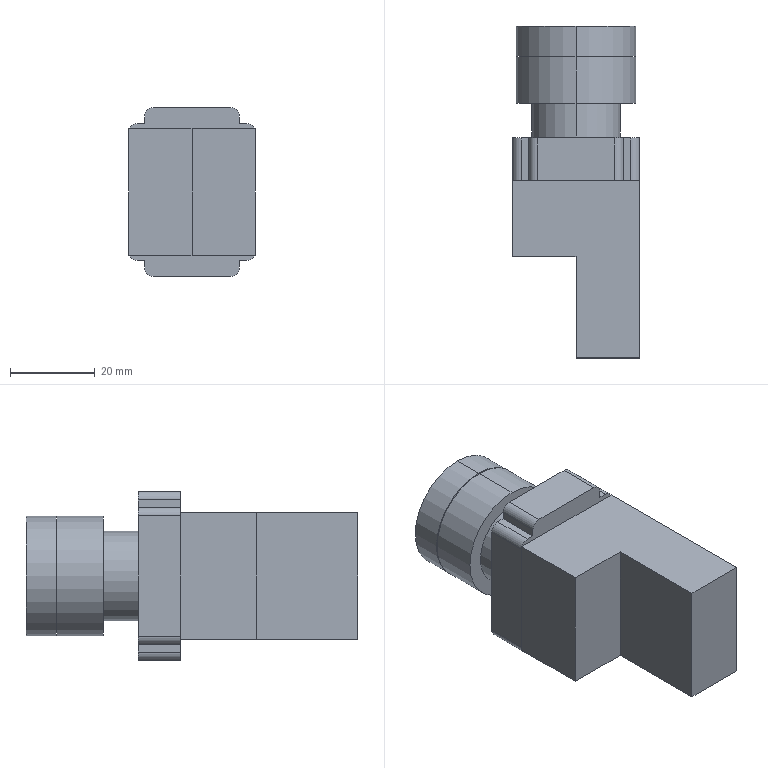Part | SolidWorks | features Boss 3, Revolution 2, Cut 1, Fillet 1 | 4 solids | 46 faces | box 30 x 78.5 x 40 mm | volume 52539 mm3 | plane 28 | cylinder 18 | commonest cylinder face diameters 4 x8 28.2 x4 21.2 x2 25 x2 25.4 x2
STEP:
#1=CARTESIAN_POINT('',(0.,8.2,-10.6));
#2=VERTEX_POINT('',#1);
#3=CARTESIAN_POINT('',(0.,8.2,10.6));
#4=VERTEX_POINT('',#3);
#5=CARTESIAN_POINT('',(0.,8.2,0.));
#6=DIRECTION('',(0.,-1.,0.));
#7=DIRECTION('',(0.,0.,-1.));
#8=AXIS2_PLACEMENT_3D('',#5,#6,#7);
#9=CIRCLE('',#8,10.6);
#10=EDGE_CURVE('',#2,#4,#9,.T.);
#11=ORIENTED_EDGE('',*,*,#10,.T.);
#12=CARTESIAN_POINT('',(0.,0.,10.6));
#13=VERTEX_POINT('',#12);
#14=CARTESIAN_POINT('',(0.,0.,10.6));
#15=DIRECTION('',(0.,-1.,0.));
#16=VECTOR('',#15,1000.);
#17=LINE('',#14,#16);
#18=EDGE_CURVE('',#4,#13,#17,.T.);
#19=ORIENTED_EDGE('',*,*,#18,.T.);
#20=CARTESIAN_POINT('',(0.,0.,-10.6));
#21=VERTEX_POINT('',#20);
#22=CARTESIAN_POINT('',(0.,0.,0.));
#23=DIRECTION('',(0.,-1.,0.));
#24=DIRECTION('',(0.,0.,-1.));
#25=AXIS2_PLACEMENT_3D('',#22,#23,#24);
#26=CIRCLE('',#25,10.6);
#27=EDGE_CURVE('',#21,#13,#26,.T.);
#28=ORIENTED_EDGE('',*,*,#27,.F.);
#29=CARTESIAN_POINT('',(0.,0.,-10.6));
#30=DIRECTION('',(0.,-1.,0.));
#31=VECTOR('',#30,1000.);
#32=LINE('',#29,#31);
#33=EDGE_CURVE('',#2,#21,#32,.T.);
#34=ORIENTED_EDGE('',*,*,#33,.F.);
#35=EDGE_LOOP('',(#11,#19,#28,#34));
#36=FACE_OUTER_BOUND('',#35,.T.);
#37=CARTESIAN_POINT('',(0.,0.,0.));
#38=DIRECTION('',(0.,-1.,0.));
#39=DIRECTION('',(0.,0.,-1.));
#40=AXIS2_PLACEMENT_3D('',#37,#38,#39);
#41=CYLINDRICAL_SURFACE('',#40,10.6);
#42=ADVANCED_FACE('',(#36),#41,.T.);
#43=CARTESIAN_POINT('',(0.,19.2,-14.1));
#44=VERTEX_POINT('',#43);
#45=CARTESIAN_POINT('',(0.,19.2,14.1));
#46=VERTEX_POINT('',#45);
#47=CARTESIAN_POINT('',(0.,19.2,0.));
#48=DIRECTION('',(0.,-1.,0.));
#49=DIRECTION('',(0.,0.,-1.));
#50=AXIS2_PLACEMENT_3D('',#47,#48,#49);
#51=CIRCLE('',#50,14.1);
#52=EDGE_CURVE('',#44,#46,#51,.T.);
#53=ORIENTED_EDGE('',*,*,#52,.T.);
#54=CARTESIAN_POINT('',(0.,8.2,14.1));
#55=VERTEX_POINT('',#54);
#56=CARTESIAN_POINT('',(0.,0.,14.1));
#57=DIRECTION('',(0.,-1.,0.));
#58=VECTOR('',#57,1000.);
#59=LINE('',#56,#58);
#60=EDGE_CURVE('',#46,#55,#59,.T.);
#61=ORIENTED_EDGE('',*,*,#60,.T.);
#62=CARTESIAN_POINT('',(0.,8.2,-14.1));
#63=VERTEX_POINT('',#62);
#64=CARTESIAN_POINT('',(0.,8.2,0.));
#65=DIRECTION('',(0.,-1.,0.));
#66=DIRECTION('',(0.,0.,-1.));
#67=AXIS2_PLACEMENT_3D('',#64,#65,#66);
#68=CIRCLE('',#67,14.1);
#69=EDGE_CURVE('',#63,#55,#68,.T.);
#70=ORIENTED_EDGE('',*,*,#69,.F.);
#71=CARTESIAN_POINT('',(0.,0.,-14.1));
#72=DIRECTION('',(0.,-1.,0.));
#73=VECTOR('',#72,1000.);
#74=LINE('',#71,#73);
#75=EDGE_CURVE('',#44,#63,#74,.T.);
#76=ORIENTED_EDGE('',*,*,#75,.F.);
#77=EDGE_LOOP('',(#53,#61,#70,#76));
#78=FACE_OUTER_BOUND('',#77,.T.);
#79=CARTESIAN_POINT('',(0.,0.,0.));
#80=DIRECTION('',(0.,-1.,0.));
#81=DIRECTION('',(0.,0.,-1.));
#82=AXIS2_PLACEMENT_3D('',#79,#80,#81);
#83=CYLINDRICAL_SURFACE('',#82,14.1);
#84=ADVANCED_FACE('',(#78),#83,.T.);
#85=CARTESIAN_POINT('',(0.,26.5,-12.5));
#86=VERTEX_POINT('',#85);
#87=CARTESIAN_POINT('',(0.,26.5,12.5));
#88=VERTEX_POINT('',#87);
#89=CARTESIAN_POINT('',(0.,26.5,0.));
#90=DIRECTION('',(0.,-1.,0.));
#91=DIRECTION('',(0.,0.,-1.));
#92=AXIS2_PLACEMENT_3D('',#89,#90,#91);
#93=CIRCLE('',#92,12.5);
#94=EDGE_CURVE('',#86,#88,#93,.T.);
#95=ORIENTED_EDGE('',*,*,#94,.T.);
#96=CARTESIAN_POINT('',(0.,19.2,12.5));
#97=VERTEX_POINT('',#96);
#98=CARTESIAN_POINT('',(0.,0.,12.5));
#99=DIRECTION('',(0.,-1.,0.));
#100=VECTOR('',#99,1000.);
#101=LINE('',#98,#100);
#102=EDGE_CURVE('',#88,#97,#101,.T.);
#103=ORIENTED_EDGE('',*,*,#102,.T.);
#104=CARTESIAN_POINT('',(0.,19.2,-12.5));
#105=VERTEX_POINT('',#104);
#106=CARTESIAN_POINT('',(0.,19.2,0.));
#107=DIRECTION('',(0.,-1.,0.));
#108=DIRECTION('',(0.,0.,-1.));
#109=AXIS2_PLACEMENT_3D('',#106,#107,#108);
#110=CIRCLE('',#109,12.5);
#111=EDGE_CURVE('',#105,#97,#110,.T.);
#112=ORIENTED_EDGE('',*,*,#111,.F.);
#113=CARTESIAN_POINT('',(0.,0.,-12.5));
#114=DIRECTION('',(0.,-1.,0.));
#115=VECTOR('',#114,1000.);
#116=LINE('',#113,#115);
#117=EDGE_CURVE('',#86,#105,#116,.T.);
#118=ORIENTED_EDGE('',*,*,#117,.F.);
#119=EDGE_LOOP('',(#95,#103,#112,#118));
#120=FACE_OUTER_BOUND('',#119,.T.);
#121=CARTESIAN_POINT('',(0.,0.,0.));
#122=DIRECTION('',(0.,-1.,0.));
#123=DIRECTION('',(0.,0.,-1.));
#124=AXIS2_PLACEMENT_3D('',#121,#122,#123);
#125=CYLINDRICAL_SURFACE('',#124,12.5);
#126=ADVANCED_FACE('',(#120),#125,.T.);
#127=ORIENTED_EDGE('',*,*,#27,.T.);
#128=CARTESIAN_POINT('',(0.,0.,0.));
#129=DIRECTION('',(0.,-1.,0.));
#130=DIRECTION('',(0.,0.,-1.));
#131=AXIS2_PLACEMENT_3D('',#128,#129,#130);
#132=CIRCLE('',#131,10.6);
#133=EDGE_CURVE('',#13,#21,#132,.T.);
#134=ORIENTED_EDGE('',*,*,#133,.T.);
#135=EDGE_LOOP('',(#127,#134));
#136=FACE_OUTER_BOUND('',#135,.T.);
#137=CARTESIAN_POINT('',(10.6,0.,0.));
#138=DIRECTION('',(0.,-1.,0.));
#139=DIRECTION('',(0.,0.,-1.));
#140=AXIS2_PLACEMENT_3D('',#137,#138,#139);
#141=PLANE('',#140);
#142=ADVANCED_FACE('',(#136),#141,.T.);
#143=ORIENTED_EDGE('',*,*,#94,.F.);
#144=CARTESIAN_POINT('',(0.,26.5,0.));
#145=DIRECTION('',(0.,-1.,0.));
#146=DIRECTION('',(0.,0.,-1.));
#147=AXIS2_PLACEMENT_3D('',#144,#145,#146);
#148=CIRCLE('',#147,12.5);
#149=EDGE_CURVE('',#88,#86,#148,.T.);
#150=ORIENTED_EDGE('',*,*,#149,.F.);
#151=EDGE_LOOP('',(#143,#150));
#152=FACE_OUTER_BOUND('',#151,.T.);
#153=CARTESIAN_POINT('',(0.,26.5,0.));
#154=DIRECTION('',(0.,1.,0.));
#155=DIRECTION('',(0.,0.,1.));
#156=AXIS2_PLACEMENT_3D('',#153,#154,#155);
#157=PLANE('',#156);
#158=ADVANCED_FACE('',(#152),#157,.T.);
#159=ORIENTED_EDGE('',*,*,#102,.F.);
#160=ORIENTED_EDGE('',*,*,#149,.T.);
#161=ORIENTED_EDGE('',*,*,#117,.T.);
#162=CARTESIAN_POINT('',(0.,19.2,0.));
#163=DIRECTION('',(0.,-1.,0.));
#164=DIRECTION('',(0.,0.,-1.));
#165=AXIS2_PLACEMENT_3D('',#162,#163,#164);
#166=CIRCLE('',#165,12.5);
#167=EDGE_CURVE('',#97,#105,#166,.T.);
#168=ORIENTED_EDGE('',*,*,#167,.F.);
#169=EDGE_LOOP('',(#159,#160,#161,#168));
#170=FACE_OUTER_BOUND('',#169,.T.);
#171=CARTESIAN_POINT('',(0.,0.,0.));
#172=DIRECTION('',(0.,-1.,0.));
#173=DIRECTION('',(0.,0.,-1.));
#174=AXIS2_PLACEMENT_3D('',#171,#172,#173);
#175=CYLINDRICAL_SURFACE('',#174,12.5);
#176=ADVANCED_FACE('',(#170),#175,.T.);
#177=ORIENTED_EDGE('',*,*,#111,.T.);
#178=ORIENTED_EDGE('',*,*,#167,.T.);
#179=EDGE_LOOP('',(#177,#178));
#180=FACE_BOUND('',#179,.T.);
#181=ORIENTED_EDGE('',*,*,#52,.F.);
#182=CARTESIAN_POINT('',(0.,19.2,0.));
#183=DIRECTION('',(0.,-1.,0.));
#184=DIRECTION('',(0.,0.,-1.));
#185=AXIS2_PLACEMENT_3D('',#182,#183,#184);
#186=CIRCLE('',#185,14.1);
#187=EDGE_CURVE('',#46,#44,#186,.T.);
#188=ORIENTED_EDGE('',*,*,#187,.F.);
#189=EDGE_LOOP('',(#181,#188));
#190=FACE_OUTER_BOUND('',#189,.T.);
#191=CARTESIAN_POINT('',(12.5,19.2,0.));
#192=DIRECTION('',(0.,1.,0.));
#193=DIRECTION('',(0.,0.,1.));
#194=AXIS2_PLACEMENT_3D('',#191,#192,#193);
#195=PLANE('',#194);
#196=ADVANCED_FACE('',(#180,#190),#195,.T.);
#197=ORIENTED_EDGE('',*,*,#60,.F.);
#198=ORIENTED_EDGE('',*,*,#187,.T.);
#199=ORIENTED_EDGE('',*,*,#75,.T.);
#200=CARTESIAN_POINT('',(0.,8.2,0.));
#201=DIRECTION('',(0.,-1.,0.));
#202=DIRECTION('',(0.,0.,-1.));
#203=AXIS2_PLACEMENT_3D('',#200,#201,#202);
#204=CIRCLE('',#203,14.1);
#205=EDGE_CURVE('',#55,#63,#204,.T.);
#206=ORIENTED_EDGE('',*,*,#205,.F.);
#207=EDGE_LOOP('',(#197,#198,#199,#206));
#208=FACE_OUTER_BOUND('',#207,.T.);
#209=CARTESIAN_POINT('',(0.,0.,0.));
#210=DIRECTION('',(0.,-1.,0.));
#211=DIRECTION('',(0.,0.,-1.));
#212=AXIS2_PLACEMENT_3D('',#209,#210,#211);
#213=CYLINDRICAL_SURFACE('',#212,14.1);
#214=ADVANCED_FACE('',(#208),#213,.T.);
#215=ORIENTED_EDGE('',*,*,#69,.T.);
#216=ORIENTED_EDGE('',*,*,#205,.T.);
#217=EDGE_LOOP('',(#215,#216));
#218=FACE_OUTER_BOUND('',#217,.T.);
#219=ORIENTED_EDGE('',*,*,#10,.F.);
#220=CARTESIAN_POINT('',(0.,8.2,0.));
#221=DIRECTION('',(0.,-1.,0.));
#222=DIRECTION('',(0.,0.,-1.));
#223=AXIS2_PLACEMENT_3D('',#220,#221,#222);
#224=CIRCLE('',#223,10.6);
#225=EDGE_CURVE('',#4,#2,#224,.T.);
#226=ORIENTED_EDGE('',*,*,#225,.F.);
#227=EDGE_LOOP('',(#219,#226));
#228=FACE_BOUND('',#227,.T.);
#229=CARTESIAN_POINT('',(14.1,8.2,0.));
#230=DIRECTION('',(0.,-1.,0.));
#231=DIRECTION('',(0.,0.,-1.));
#232=AXIS2_PLACEMENT_3D('',#229,#230,#231);
#233=PLANE('',#232);
#234=ADVANCED_FACE('',(#218,#228),#233,.T.);
#235=ORIENTED_EDGE('',*,*,#18,.F.);
#236=ORIENTED_EDGE('',*,*,#225,.T.);
#237=ORIENTED_EDGE('',*,*,#33,.T.);
#238=ORIENTED_EDGE('',*,*,#133,.F.);
#239=EDGE_LOOP('',(#235,#236,#237,#238));
#240=FACE_OUTER_BOUND('',#239,.T.);
#241=CARTESIAN_POINT('',(0.,0.,0.));
#242=DIRECTION('',(0.,-1.,0.));
#243=DIRECTION('',(0.,0.,-1.));
#244=AXIS2_PLACEMENT_3D('',#241,#242,#243);
#245=CYLINDRICAL_SURFACE('',#244,10.6);
#246=ADVANCED_FACE('',(#240),#245,.T.);
#247=CLOSED_SHELL('',(#42,#84,#126,#142,#158,#176,#196,#214,#234,#246));
#248=MANIFOLD_SOLID_BREP('',#247);
#249=CARTESIAN_POINT('',(15.,0.,-14.2));
#250=VERTEX_POINT('',#249);
#251=CARTESIAN_POINT('',(15.,0.,14.2));
#252=VERTEX_POINT('',#251);
#253=CARTESIAN_POINT('',(15.,0.,20.));
#254=DIRECTION('',(0.,0.,1.));
#255=VECTOR('',#254,1000.);
#256=LINE('',#253,#255);
#257=EDGE_CURVE('',#250,#252,#256,.T.);
#258=ORIENTED_EDGE('',*,*,#257,.T.);
#259=CARTESIAN_POINT('',(15.,-10.,14.2));
#260=VERTEX_POINT('',#259);
#261=CARTESIAN_POINT('',(15.,-10.,14.2));
#262=DIRECTION('',(0.,-1.,0.));
#263=VECTOR('',#262,1000.);
#264=LINE('',#261,#263);
#265=EDGE_CURVE('',#252,#260,#264,.T.);
#266=ORIENTED_EDGE('',*,*,#265,.T.);
#267=CARTESIAN_POINT('',(15.,-10.,-14.2));
#268=VERTEX_POINT('',#267);
#269=CARTESIAN_POINT('',(15.,-10.,20.));
#270=DIRECTION('',(0.,0.,1.));
#271=VECTOR('',#270,1000.);
#272=LINE('',#269,#271);
#273=EDGE_CURVE('',#268,#260,#272,.T.);
#274=ORIENTED_EDGE('',*,*,#273,.F.);
#275=CARTESIAN_POINT('',(15.,-10.,-14.2));
#276=DIRECTION('',(0.,1.,0.));
#277=VECTOR('',#276,1000.);
#278=LINE('',#275,#277);
#279=EDGE_CURVE('',#268,#250,#278,.T.);
#280=ORIENTED_EDGE('',*,*,#279,.T.);
#281=EDGE_LOOP('',(#258,#266,#274,#280));
#282=FACE_OUTER_BOUND('',#281,.T.);
#283=CARTESIAN_POINT('',(15.,-10.,20.));
#284=DIRECTION('',(-1.,0.,0.));
#285=DIRECTION('',(0.,0.,1.));
#286=AXIS2_PLACEMENT_3D('',#283,#284,#285);
#287=PLANE('',#286);
#288=ADVANCED_FACE('',(#282),#287,.F.);
#289=CARTESIAN_POINT('',(9.2,0.,20.));
#290=VERTEX_POINT('',#289);
#291=CARTESIAN_POINT('',(-9.2,0.,20.));
#292=VERTEX_POINT('',#291);
#293=CARTESIAN_POINT('',(15.,0.,20.));
#294=DIRECTION('',(-1.,0.,0.));
#295=VECTOR('',#294,1000.);
#296=LINE('',#293,#295);
#297=EDGE_CURVE('',#290,#292,#296,.T.);
#298=ORIENTED_EDGE('',*,*,#297,.T.);
#299=CARTESIAN_POINT('',(-9.2,-10.,20.));
#300=VERTEX_POINT('',#299);
#301=CARTESIAN_POINT('',(-9.2,-10.,20.));
#302=DIRECTION('',(0.,-1.,0.));
#303=VECTOR('',#302,1000.);
#304=LINE('',#301,#303);
#305=EDGE_CURVE('',#292,#300,#304,.T.);
#306=ORIENTED_EDGE('',*,*,#305,.T.);
#307=CARTESIAN_POINT('',(9.2,-10.,20.));
#308=VERTEX_POINT('',#307);
#309=CARTESIAN_POINT('',(15.,-10.,20.));
#310=DIRECTION('',(-1.,0.,0.));
#311=VECTOR('',#310,1000.);
#312=LINE('',#309,#311);
#313=EDGE_CURVE('',#308,#300,#312,.T.);
#314=ORIENTED_EDGE('',*,*,#313,.F.);
#315=CARTESIAN_POINT('',(9.2,-10.,20.));
#316=DIRECTION('',(0.,1.,0.));
#317=VECTOR('',#316,1000.);
#318=LINE('',#315,#317);
#319=EDGE_CURVE('',#308,#290,#318,.T.);
#320=ORIENTED_EDGE('',*,*,#319,.T.);
#321=EDGE_LOOP('',(#298,#306,#314,#320));
#322=FACE_OUTER_BOUND('',#321,.T.);
#323=CARTESIAN_POINT('',(15.,-10.,20.));
#324=DIRECTION('',(0.,0.,-1.));
#325=DIRECTION('',(-1.,0.,0.));
#326=AXIS2_PLACEMENT_3D('',#323,#324,#325);
#327=PLANE('',#326);
#328=ADVANCED_FACE('',(#322),#327,.F.);
#329=CARTESIAN_POINT('',(-15.,-10.,14.2));
#330=VERTEX_POINT('',#329);
#331=CARTESIAN_POINT('',(-15.,-10.,-14.2));
#332=VERTEX_POINT('',#331);
#333=CARTESIAN_POINT('',(-15.,-10.,20.));
#334=DIRECTION('',(0.,0.,-1.));
#335=VECTOR('',#334,1000.);
#336=LINE('',#333,#335);
#337=EDGE_CURVE('',#330,#332,#336,.T.);
#338=ORIENTED_EDGE('',*,*,#337,.F.);
#339=CARTESIAN_POINT('',(-15.,0.,14.2));
#340=VERTEX_POINT('',#339);
#341=CARTESIAN_POINT('',(-15.,-10.,14.2));
#342=DIRECTION('',(0.,1.,0.));
#343=VECTOR('',#342,1000.);
#344=LINE('',#341,#343);
#345=EDGE_CURVE('',#330,#340,#344,.T.);
#346=ORIENTED_EDGE('',*,*,#345,.T.);
#347=CARTESIAN_POINT('',(-15.,0.,-14.2));
#348=VERTEX_POINT('',#347);
#349=CARTESIAN_POINT('',(-15.,0.,20.));
#350=DIRECTION('',(0.,0.,-1.));
#351=VECTOR('',#350,1000.);
#352=LINE('',#349,#351);
#353=EDGE_CURVE('',#340,#348,#352,.T.);
#354=ORIENTED_EDGE('',*,*,#353,.T.);
#355=CARTESIAN_POINT('',(-15.,-10.,-14.2));
#356=DIRECTION('',(0.,-1.,0.));
#357=VECTOR('',#356,1000.);
#358=LINE('',#355,#357);
#359=EDGE_CURVE('',#348,#332,#358,.T.);
#360=ORIENTED_EDGE('',*,*,#359,.T.);
#361=EDGE_LOOP('',(#338,#346,#354,#360));
#362=FACE_OUTER_BOUND('',#361,.T.);
#363=CARTESIAN_POINT('',(-15.,-10.,20.));
#364=DIRECTION('',(1.,0.,0.));
#365=DIRECTION('',(0.,0.,-1.));
#366=AXIS2_PLACEMENT_3D('',#363,#364,#365);
#367=PLANE('',#366);
#368=ADVANCED_FACE('',(#362),#367,.F.);
#369=CARTESIAN_POINT('',(-9.2,0.,-20.));
#370=VERTEX_POINT('',#369);
#371=CARTESIAN_POINT('',(9.2,0.,-20.));
#372=VERTEX_POINT('',#371);
#373=CARTESIAN_POINT('',(15.,0.,-20.));
#374=DIRECTION('',(1.,0.,0.));
#375=VECTOR('',#374,1000.);
#376=LINE('',#373,#375);
#377=EDGE_CURVE('',#370,#372,#376,.T.);
#378=ORIENTED_EDGE('',*,*,#377,.T.);
#379=CARTESIAN_POINT('',(9.2,-10.,-20.));
#380=VERTEX_POINT('',#379);
#381=CARTESIAN_POINT('',(9.2,-10.,-20.));
#382=DIRECTION('',(0.,-1.,0.));
#383=VECTOR('',#382,1000.);
#384=LINE('',#381,#383);
#385=EDGE_CURVE('',#372,#380,#384,.T.);
#386=ORIENTED_EDGE('',*,*,#385,.T.);
#387=CARTESIAN_POINT('',(-9.2,-10.,-20.));
#388=VERTEX_POINT('',#387);
#389=CARTESIAN_POINT('',(15.,-10.,-20.));
#390=DIRECTION('',(1.,0.,0.));
#391=VECTOR('',#390,1000.);
#392=LINE('',#389,#391);
#393=EDGE_CURVE('',#388,#380,#392,.T.);
#394=ORIENTED_EDGE('',*,*,#393,.F.);
#395=CARTESIAN_POINT('',(-9.2,-10.,-20.));
#396=DIRECTION('',(0.,1.,0.));
#397=VECTOR('',#396,1000.);
#398=LINE('',#395,#397);
#399=EDGE_CURVE('',#388,#370,#398,.T.);
#400=ORIENTED_EDGE('',*,*,#399,.T.);
#401=EDGE_LOOP('',(#378,#386,#394,#400));
#402=FACE_OUTER_BOUND('',#401,.T.);
#403=CARTESIAN_POINT('',(15.,-10.,-20.));
#404=DIRECTION('',(0.,0.,1.));
#405=DIRECTION('',(1.,0.,0.));
#406=AXIS2_PLACEMENT_3D('',#403,#404,#405);
#407=PLANE('',#406);
#408=ADVANCED_FACE('',(#402),#407,.F.);
#409=CARTESIAN_POINT('',(-13.,-10.,16.2));
#410=VERTEX_POINT('',#409);
#411=CARTESIAN_POINT('',(-11.2,-10.,16.2));
#412=VERTEX_POINT('',#411);
#413=CARTESIAN_POINT('',(-15.,-10.,16.2));
#414=DIRECTION('',(1.,0.,0.));
#415=VECTOR('',#414,1000.);
#416=LINE('',#413,#415);
#417=EDGE_CURVE('',#410,#412,#416,.T.);
#418=ORIENTED_EDGE('',*,*,#417,.F.);
#419=CARTESIAN_POINT('',(-13.,-10.,14.2));
#420=DIRECTION('',(0.,-1.,0.));
#421=DIRECTION('',(0.,0.,1.));
#422=AXIS2_PLACEMENT_3D('',#419,#420,#421);
#423=CIRCLE('',#422,2.);
#424=EDGE_CURVE('',#410,#330,#423,.T.);
#425=ORIENTED_EDGE('',*,*,#424,.T.);
#426=ORIENTED_EDGE('',*,*,#337,.T.);
#427=CARTESIAN_POINT('',(-13.,-10.,-16.2));
#428=VERTEX_POINT('',#427);
#429=CARTESIAN_POINT('',(-13.,-10.,-14.2));
#430=DIRECTION('',(0.,-1.,0.));
#431=DIRECTION('',(0.,0.,1.));
#432=AXIS2_PLACEMENT_3D('',#429,#430,#431);
#433=CIRCLE('',#432,2.);
#434=EDGE_CURVE('',#332,#428,#433,.T.);
#435=ORIENTED_EDGE('',*,*,#434,.T.);
#436=CARTESIAN_POINT('',(-11.2,-10.,-16.2));
#437=VERTEX_POINT('',#436);
#438=CARTESIAN_POINT('',(-15.,-10.,-16.2));
#439=DIRECTION('',(-1.,0.,0.));
#440=VECTOR('',#439,1000.);
#441=LINE('',#438,#440);
#442=EDGE_CURVE('',#437,#428,#441,.T.);
#443=ORIENTED_EDGE('',*,*,#442,.F.);
#444=CARTESIAN_POINT('',(-11.2,-10.,-18.));
#445=VERTEX_POINT('',#444);
#446=CARTESIAN_POINT('',(-11.2,-10.,-20.));
#447=DIRECTION('',(0.,0.,1.));
#448=VECTOR('',#447,1000.);
#449=LINE('',#446,#448);
#450=EDGE_CURVE('',#445,#437,#449,.T.);
#451=ORIENTED_EDGE('',*,*,#450,.F.);
#452=CARTESIAN_POINT('',(-9.2,-10.,-18.));
#453=DIRECTION('',(0.,-1.,0.));
#454=DIRECTION('',(0.,0.,1.));
#455=AXIS2_PLACEMENT_3D('',#452,#453,#454);
#456=CIRCLE('',#455,2.);
#457=EDGE_CURVE('',#445,#388,#456,.T.);
#458=ORIENTED_EDGE('',*,*,#457,.T.);
#459=ORIENTED_EDGE('',*,*,#393,.T.);
#460=CARTESIAN_POINT('',(11.2,-10.,-18.));
#461=VERTEX_POINT('',#460);
#462=CARTESIAN_POINT('',(9.2,-10.,-18.));
#463=DIRECTION('',(0.,-1.,0.));
#464=DIRECTION('',(0.,0.,1.));
#465=AXIS2_PLACEMENT_3D('',#462,#463,#464);
#466=CIRCLE('',#465,2.);
#467=EDGE_CURVE('',#380,#461,#466,.T.);
#468=ORIENTED_EDGE('',*,*,#467,.T.);
#469=CARTESIAN_POINT('',(11.2,-10.,-16.2));
#470=VERTEX_POINT('',#469);
#471=CARTESIAN_POINT('',(11.2,-10.,-20.));
#472=DIRECTION('',(0.,0.,-1.));
#473=VECTOR('',#472,1000.);
#474=LINE('',#471,#473);
#475=EDGE_CURVE('',#470,#461,#474,.T.);
#476=ORIENTED_EDGE('',*,*,#475,.F.);
#477=CARTESIAN_POINT('',(13.,-10.,-16.2));
#478=VERTEX_POINT('',#477);
#479=CARTESIAN_POINT('',(15.,-10.,-16.2));
#480=DIRECTION('',(-1.,0.,0.));
#481=VECTOR('',#480,1000.);
#482=LINE('',#479,#481);
#483=EDGE_CURVE('',#478,#470,#482,.T.);
#484=ORIENTED_EDGE('',*,*,#483,.F.);
#485=CARTESIAN_POINT('',(13.,-10.,-14.2));
#486=DIRECTION('',(0.,-1.,0.));
#487=DIRECTION('',(0.,0.,1.));
#488=AXIS2_PLACEMENT_3D('',#485,#486,#487);
#489=CIRCLE('',#488,2.);
#490=EDGE_CURVE('',#478,#268,#489,.T.);
#491=ORIENTED_EDGE('',*,*,#490,.T.);
#492=ORIENTED_EDGE('',*,*,#273,.T.);
#493=CARTESIAN_POINT('',(13.,-10.,16.2));
#494=VERTEX_POINT('',#493);
#495=CARTESIAN_POINT('',(13.,-10.,14.2));
#496=DIRECTION('',(0.,-1.,0.));
#497=DIRECTION('',(0.,0.,1.));
#498=AXIS2_PLACEMENT_3D('',#495,#496,#497);
#499=CIRCLE('',#498,2.);
#500=EDGE_CURVE('',#260,#494,#499,.T.);
#501=ORIENTED_EDGE('',*,*,#500,.T.);
#502=CARTESIAN_POINT('',(11.2,-10.,16.2));
#503=VERTEX_POINT('',#502);
#504=CARTESIAN_POINT('',(15.,-10.,16.2));
#505=DIRECTION('',(1.,0.,0.));
#506=VECTOR('',#505,1000.);
#507=LINE('',#504,#506);
#508=EDGE_CURVE('',#503,#494,#507,.T.);
#509=ORIENTED_EDGE('',*,*,#508,.F.);
#510=CARTESIAN_POINT('',(11.2,-10.,18.));
#511=VERTEX_POINT('',#510);
#512=CARTESIAN_POINT('',(11.2,-10.,20.));
#513=DIRECTION('',(0.,0.,-1.));
#514=VECTOR('',#513,1000.);
#515=LINE('',#512,#514);
#516=EDGE_CURVE('',#511,#503,#515,.T.);
#517=ORIENTED_EDGE('',*,*,#516,.F.);
#518=CARTESIAN_POINT('',(9.2,-10.,18.));
#519=DIRECTION('',(0.,-1.,0.));
#520=DIRECTION('',(0.,0.,1.));
#521=AXIS2_PLACEMENT_3D('',#518,#519,#520);
#522=CIRCLE('',#521,2.);
#523=EDGE_CURVE('',#511,#308,#522,.T.);
#524=ORIENTED_EDGE('',*,*,#523,.T.);
#525=ORIENTED_EDGE('',*,*,#313,.T.);
#526=CARTESIAN_POINT('',(-11.2,-10.,18.));
#527=VERTEX_POINT('',#526);
#528=CARTESIAN_POINT('',(-9.2,-10.,18.));
#529=DIRECTION('',(0.,-1.,0.));
#530=DIRECTION('',(0.,0.,1.));
#531=AXIS2_PLACEMENT_3D('',#528,#529,#530);
#532=CIRCLE('',#531,2.);
#533=EDGE_CURVE('',#300,#527,#532,.T.);
#534=ORIENTED_EDGE('',*,*,#533,.T.);
#535=CARTESIAN_POINT('',(-11.2,-10.,20.));
#536=DIRECTION('',(0.,0.,1.));
#537=VECTOR('',#536,1000.);
#538=LINE('',#535,#537);
#539=EDGE_CURVE('',#412,#527,#538,.T.);
#540=ORIENTED_EDGE('',*,*,#539,.F.);
#541=EDGE_LOOP('',(#418,#425,#426,#435,#443,#451,#458,#459,#468,#476,#484,#491,#492,#501,#509,#517,#524,#525,#534,#540));
#542=FACE_OUTER_BOUND('',#541,.T.);
#543=CARTESIAN_POINT('',(15.,-10.,20.));
#544=DIRECTION('',(0.,1.,0.));
#545=DIRECTION('',(0.,0.,1.));
#546=AXIS2_PLACEMENT_3D('',#543,#544,#545);
#547=PLANE('',#546);
#548=ADVANCED_FACE('',(#542),#547,.F.);
#549=ORIENTED_EDGE('',*,*,#353,.F.);
#550=CARTESIAN_POINT('',(-13.,0.,16.2));
#551=VERTEX_POINT('',#550);
#552=CARTESIAN_POINT('',(-13.,0.,14.2));
#553=DIRECTION('',(0.,1.,0.));
#554=DIRECTION('',(0.,0.,1.));
#555=AXIS2_PLACEMENT_3D('',#552,#553,#554);
#556=CIRCLE('',#555,2.);
#557=EDGE_CURVE('',#340,#551,#556,.T.);
#558=ORIENTED_EDGE('',*,*,#557,.T.);
#559=CARTESIAN_POINT('',(-11.2,0.,16.2));
#560=VERTEX_POINT('',#559);
#561=CARTESIAN_POINT('',(-15.,0.,16.2));
#562=DIRECTION('',(-1.,0.,0.));
#563=VECTOR('',#562,1000.);
#564=LINE('',#561,#563);
#565=EDGE_CURVE('',#560,#551,#564,.T.);
#566=ORIENTED_EDGE('',*,*,#565,.F.);
#567=CARTESIAN_POINT('',(-11.2,0.,18.));
#568=VERTEX_POINT('',#567);
#569=CARTESIAN_POINT('',(-11.2,0.,20.));
#570=DIRECTION('',(0.,0.,-1.));
#571=VECTOR('',#570,1000.);
#572=LINE('',#569,#571);
#573=EDGE_CURVE('',#568,#560,#572,.T.);
#574=ORIENTED_EDGE('',*,*,#573,.F.);
#575=CARTESIAN_POINT('',(-9.2,0.,18.));
#576=DIRECTION('',(0.,1.,0.));
#577=DIRECTION('',(0.,0.,1.));
#578=AXIS2_PLACEMENT_3D('',#575,#576,#577);
#579=CIRCLE('',#578,2.);
#580=EDGE_CURVE('',#568,#292,#579,.T.);
#581=ORIENTED_EDGE('',*,*,#580,.T.);
#582=ORIENTED_EDGE('',*,*,#297,.F.);
#583=CARTESIAN_POINT('',(11.2,0.,18.));
#584=VERTEX_POINT('',#583);
#585=CARTESIAN_POINT('',(9.2,0.,18.));
#586=DIRECTION('',(0.,1.,0.));
#587=DIRECTION('',(0.,0.,1.));
#588=AXIS2_PLACEMENT_3D('',#585,#586,#587);
#589=CIRCLE('',#588,2.);
#590=EDGE_CURVE('',#290,#584,#589,.T.);
#591=ORIENTED_EDGE('',*,*,#590,.T.);
#592=CARTESIAN_POINT('',(11.2,0.,16.2));
#593=VERTEX_POINT('',#592);
#594=CARTESIAN_POINT('',(11.2,0.,20.));
#595=DIRECTION('',(0.,0.,1.));
#596=VECTOR('',#595,1000.);
#597=LINE('',#594,#596);
#598=EDGE_CURVE('',#593,#584,#597,.T.);
#599=ORIENTED_EDGE('',*,*,#598,.F.);
#600=CARTESIAN_POINT('',(13.,0.,16.2));
#601=VERTEX_POINT('',#600);
#602=CARTESIAN_POINT('',(15.,0.,16.2));
#603=DIRECTION('',(-1.,0.,0.));
#604=VECTOR('',#603,1000.);
#605=LINE('',#602,#604);
#606=EDGE_CURVE('',#601,#593,#605,.T.);
#607=ORIENTED_EDGE('',*,*,#606,.F.);
#608=CARTESIAN_POINT('',(13.,0.,14.2));
#609=DIRECTION('',(0.,1.,0.));
#610=DIRECTION('',(0.,0.,1.));
#611=AXIS2_PLACEMENT_3D('',#608,#609,#610);
#612=CIRCLE('',#611,2.);
#613=EDGE_CURVE('',#601,#252,#612,.T.);
#614=ORIENTED_EDGE('',*,*,#613,.T.);
#615=ORIENTED_EDGE('',*,*,#257,.F.);
#616=CARTESIAN_POINT('',(13.,0.,-16.2));
#617=VERTEX_POINT('',#616);
#618=CARTESIAN_POINT('',(13.,0.,-14.2));
#619=DIRECTION('',(0.,1.,0.));
#620=DIRECTION('',(0.,0.,1.));
#621=AXIS2_PLACEMENT_3D('',#618,#619,#620);
#622=CIRCLE('',#621,2.);
#623=EDGE_CURVE('',#250,#617,#622,.T.);
#624=ORIENTED_EDGE('',*,*,#623,.T.);
#625=CARTESIAN_POINT('',(11.2,0.,-16.2));
#626=VERTEX_POINT('',#625);
#627=CARTESIAN_POINT('',(15.,0.,-16.2));
#628=DIRECTION('',(1.,0.,0.));
#629=VECTOR('',#628,1000.);
#630=LINE('',#627,#629);
#631=EDGE_CURVE('',#626,#617,#630,.T.);
#632=ORIENTED_EDGE('',*,*,#631,.F.);
#633=CARTESIAN_POINT('',(11.2,0.,-18.));
#634=VERTEX_POINT('',#633);
#635=CARTESIAN_POINT('',(11.2,0.,-20.));
#636=DIRECTION('',(0.,0.,1.));
#637=VECTOR('',#636,1000.);
#638=LINE('',#635,#637);
#639=EDGE_CURVE('',#634,#626,#638,.T.);
#640=ORIENTED_EDGE('',*,*,#639,.F.);
#641=CARTESIAN_POINT('',(9.2,0.,-18.));
#642=DIRECTION('',(0.,1.,0.));
#643=DIRECTION('',(0.,0.,1.));
#644=AXIS2_PLACEMENT_3D('',#641,#642,#643);
#645=CIRCLE('',#644,2.);
#646=EDGE_CURVE('',#634,#372,#645,.T.);
#647=ORIENTED_EDGE('',*,*,#646,.T.);
#648=ORIENTED_EDGE('',*,*,#377,.F.);
#649=CARTESIAN_POINT('',(-11.2,0.,-18.));
#650=VERTEX_POINT('',#649);
#651=CARTESIAN_POINT('',(-9.2,0.,-18.));
#652=DIRECTION('',(0.,1.,0.));
#653=DIRECTION('',(0.,0.,1.));
#654=AXIS2_PLACEMENT_3D('',#651,#652,#653);
#655=CIRCLE('',#654,2.);
#656=EDGE_CURVE('',#370,#650,#655,.T.);
#657=ORIENTED_EDGE('',*,*,#656,.T.);
#658=CARTESIAN_POINT('',(-11.2,0.,-16.2));
#659=VERTEX_POINT('',#658);
#660=CARTESIAN_POINT('',(-11.2,0.,-20.));
#661=DIRECTION('',(0.,0.,-1.));
#662=VECTOR('',#661,1000.);
#663=LINE('',#660,#662);
#664=EDGE_CURVE('',#659,#650,#663,.T.);
#665=ORIENTED_EDGE('',*,*,#664,.F.);
#666=CARTESIAN_POINT('',(-13.,0.,-16.2));
#667=VERTEX_POINT('',#666);
#668=CARTESIAN_POINT('',(-15.,0.,-16.2));
#669=DIRECTION('',(1.,0.,0.));
#670=VECTOR('',#669,1000.);
#671=LINE('',#668,#670);
#672=EDGE_CURVE('',#667,#659,#671,.T.);
#673=ORIENTED_EDGE('',*,*,#672,.F.);
#674=CARTESIAN_POINT('',(-13.,0.,-14.2));
#675=DIRECTION('',(0.,1.,0.));
#676=DIRECTION('',(0.,0.,1.));
#677=AXIS2_PLACEMENT_3D('',#674,#675,#676);
#678=CIRCLE('',#677,2.);
#679=EDGE_CURVE('',#667,#348,#678,.T.);
#680=ORIENTED_EDGE('',*,*,#679,.T.);
#681=EDGE_LOOP('',(#549,#558,#566,#574,#581,#582,#591,#599,#607,#614,#615,#624,#632,#640,#647,#648,#657,#665,#673,#680));
#682=FACE_OUTER_BOUND('',#681,.T.);
#683=CARTESIAN_POINT('',(15.,0.,20.));
#684=DIRECTION('',(0.,1.,0.));
#685=DIRECTION('',(0.,0.,1.));
#686=AXIS2_PLACEMENT_3D('',#683,#684,#685);
#687=PLANE('',#686);
#688=ADVANCED_FACE('',(#682),#687,.T.);
#689=ORIENTED_EDGE('',*,*,#598,.T.);
#690=CARTESIAN_POINT('',(11.2,-52.001,18.));
#691=DIRECTION('',(0.,-1.,0.));
#692=VECTOR('',#691,1000.);
#693=LINE('',#690,#692);
#694=EDGE_CURVE('',#584,#511,#693,.T.);
#695=ORIENTED_EDGE('',*,*,#694,.T.);
#696=ORIENTED_EDGE('',*,*,#516,.T.);
#697=CARTESIAN_POINT('',(11.2,-52.001,16.2));
#698=DIRECTION('',(0.,1.,0.));
#699=VECTOR('',#698,1000.);
#700=LINE('',#697,#699);
#701=EDGE_CURVE('',#503,#593,#700,.T.);
#702=ORIENTED_EDGE('',*,*,#701,.T.);
#703=EDGE_LOOP('',(#689,#695,#696,#702));
#704=FACE_OUTER_BOUND('',#703,.T.);
#705=CARTESIAN_POINT('',(11.2,-52.001,20.));
#706=DIRECTION('',(-1.,0.,0.));
#707=DIRECTION('',(0.,0.,1.));
#708=AXIS2_PLACEMENT_3D('',#705,#706,#707);
#709=PLANE('',#708);
#710=ADVANCED_FACE('',(#704),#709,.F.);
#711=ORIENTED_EDGE('',*,*,#508,.T.);
#712=CARTESIAN_POINT('',(13.,-52.001,16.2));
#713=DIRECTION('',(0.,1.,0.));
#714=VECTOR('',#713,1000.);
#715=LINE('',#712,#714);
#716=EDGE_CURVE('',#494,#601,#715,.T.);
#717=ORIENTED_EDGE('',*,*,#716,.T.);
#718=ORIENTED_EDGE('',*,*,#606,.T.);
#719=ORIENTED_EDGE('',*,*,#701,.F.);
#720=EDGE_LOOP('',(#711,#717,#718,#719));
#721=FACE_OUTER_BOUND('',#720,.T.);
#722=CARTESIAN_POINT('',(15.,-52.001,16.2));
#723=DIRECTION('',(0.,0.,-1.));
#724=DIRECTION('',(-1.,0.,0.));
#725=AXIS2_PLACEMENT_3D('',#722,#723,#724);
#726=PLANE('',#725);
#727=ADVANCED_FACE('',(#721),#726,.F.);
#728=ORIENTED_EDGE('',*,*,#565,.T.);
#729=CARTESIAN_POINT('',(-13.,-52.001,16.2));
#730=DIRECTION('',(0.,-1.,0.));
#731=VECTOR('',#730,1000.);
#732=LINE('',#729,#731);
#733=EDGE_CURVE('',#551,#410,#732,.T.);
#734=ORIENTED_EDGE('',*,*,#733,.T.);
#735=ORIENTED_EDGE('',*,*,#417,.T.);
#736=CARTESIAN_POINT('',(-11.2,-52.001,16.2));
#737=DIRECTION('',(0.,1.,0.));
#738=VECTOR('',#737,1000.);
#739=LINE('',#736,#738);
#740=EDGE_CURVE('',#412,#560,#739,.T.);
#741=ORIENTED_EDGE('',*,*,#740,.T.);
#742=EDGE_LOOP('',(#728,#734,#735,#741));
#743=FACE_OUTER_BOUND('',#742,.T.);
#744=CARTESIAN_POINT('',(-15.,-52.001,16.2));
#745=DIRECTION('',(0.,0.,-1.));
#746=DIRECTION('',(-1.,0.,0.));
#747=AXIS2_PLACEMENT_3D('',#744,#745,#746);
#748=PLANE('',#747);
#749=ADVANCED_FACE('',(#743),#748,.F.);
#750=ORIENTED_EDGE('',*,*,#539,.T.);
#751=CARTESIAN_POINT('',(-11.2,-52.001,18.));
#752=DIRECTION('',(0.,1.,0.));
#753=VECTOR('',#752,1000.);
#754=LINE('',#751,#753);
#755=EDGE_CURVE('',#527,#568,#754,.T.);
#756=ORIENTED_EDGE('',*,*,#755,.T.);
#757=ORIENTED_EDGE('',*,*,#573,.T.);
#758=ORIENTED_EDGE('',*,*,#740,.F.);
#759=EDGE_LOOP('',(#750,#756,#757,#758));
#760=FACE_OUTER_BOUND('',#759,.T.);
#761=CARTESIAN_POINT('',(-11.2,-52.001,20.));
#762=DIRECTION('',(1.,0.,0.));
#763=DIRECTION('',(0.,0.,-1.));
#764=AXIS2_PLACEMENT_3D('',#761,#762,#763);
#765=PLANE('',#764);
#766=ADVANCED_FACE('',(#760),#765,.F.);
#767=ORIENTED_EDGE('',*,*,#664,.T.);
#768=CARTESIAN_POINT('',(-11.2,-52.001,-18.));
#769=DIRECTION('',(0.,-1.,0.));
#770=VECTOR('',#769,1000.);
#771=LINE('',#768,#770);
#772=EDGE_CURVE('',#650,#445,#771,.T.);
#773=ORIENTED_EDGE('',*,*,#772,.T.);
#774=ORIENTED_EDGE('',*,*,#450,.T.);
#775=CARTESIAN_POINT('',(-11.2,-52.001,-16.2));
#776=DIRECTION('',(0.,1.,0.));
#777=VECTOR('',#776,1000.);
#778=LINE('',#775,#777);
#779=EDGE_CURVE('',#437,#659,#778,.T.);
#780=ORIENTED_EDGE('',*,*,#779,.T.);
#781=EDGE_LOOP('',(#767,#773,#774,#780));
#782=FACE_OUTER_BOUND('',#781,.T.);
#783=CARTESIAN_POINT('',(-11.2,-52.001,-20.));
#784=DIRECTION('',(1.,0.,0.));
#785=DIRECTION('',(0.,0.,-1.));
#786=AXIS2_PLACEMENT_3D('',#783,#784,#785);
#787=PLANE('',#786);
#788=ADVANCED_FACE('',(#782),#787,.F.);
#789=ORIENTED_EDGE('',*,*,#442,.T.);
#790=CARTESIAN_POINT('',(-13.,-52.001,-16.2));
#791=DIRECTION('',(0.,1.,0.));
#792=VECTOR('',#791,1000.);
#793=LINE('',#790,#792);
#794=EDGE_CURVE('',#428,#667,#793,.T.);
#795=ORIENTED_EDGE('',*,*,#794,.T.);
#796=ORIENTED_EDGE('',*,*,#672,.T.);
#797=ORIENTED_EDGE('',*,*,#779,.F.);
#798=EDGE_LOOP('',(#789,#795,#796,#797));
#799=FACE_OUTER_BOUND('',#798,.T.);
#800=CARTESIAN_POINT('',(-15.,-52.001,-16.2));
#801=DIRECTION('',(0.,0.,1.));
#802=DIRECTION('',(1.,0.,0.));
#803=AXIS2_PLACEMENT_3D('',#800,#801,#802);
#804=PLANE('',#803);
#805=ADVANCED_FACE('',(#799),#804,.F.);
#806=ORIENTED_EDGE('',*,*,#631,.T.);
#807=CARTESIAN_POINT('',(13.,-52.001,-16.2));
#808=DIRECTION('',(0.,-1.,0.));
#809=VECTOR('',#808,1000.);
#810=LINE('',#807,#809);
#811=EDGE_CURVE('',#617,#478,#810,.T.);
#812=ORIENTED_EDGE('',*,*,#811,.T.);
#813=ORIENTED_EDGE('',*,*,#483,.T.);
#814=CARTESIAN_POINT('',(11.2,-52.001,-16.2));
#815=DIRECTION('',(0.,1.,0.));
#816=VECTOR('',#815,1000.);
#817=LINE('',#814,#816);
#818=EDGE_CURVE('',#470,#626,#817,.T.);
#819=ORIENTED_EDGE('',*,*,#818,.T.);
#820=EDGE_LOOP('',(#806,#812,#813,#819));
#821=FACE_OUTER_BOUND('',#820,.T.);
#822=CARTESIAN_POINT('',(15.,-52.001,-16.2));
#823=DIRECTION('',(0.,0.,1.));
#824=DIRECTION('',(1.,0.,0.));
#825=AXIS2_PLACEMENT_3D('',#822,#823,#824);
#826=PLANE('',#825);
#827=ADVANCED_FACE('',(#821),#826,.F.);
#828=ORIENTED_EDGE('',*,*,#475,.T.);
#829=CARTESIAN_POINT('',(11.2,-52.001,-18.));
#830=DIRECTION('',(0.,1.,0.));
#831=VECTOR('',#830,1000.);
#832=LINE('',#829,#831);
#833=EDGE_CURVE('',#461,#634,#832,.T.);
#834=ORIENTED_EDGE('',*,*,#833,.T.);
#835=ORIENTED_EDGE('',*,*,#639,.T.);
#836=ORIENTED_EDGE('',*,*,#818,.F.);
#837=EDGE_LOOP('',(#828,#834,#835,#836));
#838=FACE_OUTER_BOUND('',#837,.T.);
#839=CARTESIAN_POINT('',(11.2,-52.001,-20.));
#840=DIRECTION('',(-1.,0.,0.));
#841=DIRECTION('',(0.,0.,1.));
#842=AXIS2_PLACEMENT_3D('',#839,#840,#841);
#843=PLANE('',#842);
#844=ADVANCED_FACE('',(#838),#843,.F.);
#845=ORIENTED_EDGE('',*,*,#424,.F.);
#846=ORIENTED_EDGE('',*,*,#733,.F.);
#847=ORIENTED_EDGE('',*,*,#557,.F.);
#848=ORIENTED_EDGE('',*,*,#345,.F.);
#849=EDGE_LOOP('',(#845,#846,#847,#848));
#850=FACE_OUTER_BOUND('',#849,.T.);
#851=CARTESIAN_POINT('',(-13.,-10.,14.2));
#852=DIRECTION('',(0.,1.,0.));
#853=DIRECTION('',(0.,0.,1.));
#854=AXIS2_PLACEMENT_3D('',#851,#852,#853);
#855=CYLINDRICAL_SURFACE('',#854,2.);
#856=ADVANCED_FACE('',(#850),#855,.T.);
#857=ORIENTED_EDGE('',*,*,#533,.F.);
#858=ORIENTED_EDGE('',*,*,#305,.F.);
#859=ORIENTED_EDGE('',*,*,#580,.F.);
#860=ORIENTED_EDGE('',*,*,#755,.F.);
#861=EDGE_LOOP('',(#857,#858,#859,#860));
#862=FACE_OUTER_BOUND('',#861,.T.);
#863=CARTESIAN_POINT('',(-9.2,-52.001,18.));
#864=DIRECTION('',(0.,1.,0.));
#865=DIRECTION('',(0.,0.,1.));
#866=AXIS2_PLACEMENT_3D('',#863,#864,#865);
#867=CYLINDRICAL_SURFACE('',#866,2.);
#868=ADVANCED_FACE('',(#862),#867,.T.);
#869=ORIENTED_EDGE('',*,*,#523,.F.);
#870=ORIENTED_EDGE('',*,*,#694,.F.);
#871=ORIENTED_EDGE('',*,*,#590,.F.);
#872=ORIENTED_EDGE('',*,*,#319,.F.);
#873=EDGE_LOOP('',(#869,#870,#871,#872));
#874=FACE_OUTER_BOUND('',#873,.T.);
#875=CARTESIAN_POINT('',(9.2,-10.,18.));
#876=DIRECTION('',(0.,1.,0.));
#877=DIRECTION('',(0.,0.,1.));
#878=AXIS2_PLACEMENT_3D('',#875,#876,#877);
#879=CYLINDRICAL_SURFACE('',#878,2.);
#880=ADVANCED_FACE('',(#874),#879,.T.);
#881=ORIENTED_EDGE('',*,*,#500,.F.);
#882=ORIENTED_EDGE('',*,*,#265,.F.);
#883=ORIENTED_EDGE('',*,*,#613,.F.);
#884=ORIENTED_EDGE('',*,*,#716,.F.);
#885=EDGE_LOOP('',(#881,#882,#883,#884));
#886=FACE_OUTER_BOUND('',#885,.T.);
#887=CARTESIAN_POINT('',(13.,-52.001,14.2));
#888=DIRECTION('',(0.,1.,0.));
#889=DIRECTION('',(0.,0.,1.));
#890=AXIS2_PLACEMENT_3D('',#887,#888,#889);
#891=CYLINDRICAL_SURFACE('',#890,2.);
#892=ADVANCED_FACE('',(#886),#891,.T.);
#893=ORIENTED_EDGE('',*,*,#490,.F.);
#894=ORIENTED_EDGE('',*,*,#811,.F.);
#895=ORIENTED_EDGE('',*,*,#623,.F.);
#896=ORIENTED_EDGE('',*,*,#279,.F.);
#897=EDGE_LOOP('',(#893,#894,#895,#896));
#898=FACE_OUTER_BOUND('',#897,.T.);
#899=CARTESIAN_POINT('',(13.,-10.,-14.2));
#900=DIRECTION('',(0.,1.,0.));
#901=DIRECTION('',(0.,0.,1.));
#902=AXIS2_PLACEMENT_3D('',#899,#900,#901);
#903=CYLINDRICAL_SURFACE('',#902,2.);
#904=ADVANCED_FACE('',(#898),#903,.T.);
#905=ORIENTED_EDGE('',*,*,#467,.F.);
#906=ORIENTED_EDGE('',*,*,#385,.F.);
#907=ORIENTED_EDGE('',*,*,#646,.F.);
#908=ORIENTED_EDGE('',*,*,#833,.F.);
#909=EDGE_LOOP('',(#905,#906,#907,#908));
#910=FACE_OUTER_BOUND('',#909,.T.);
#911=CARTESIAN_POINT('',(9.2,-52.001,-18.));
#912=DIRECTION('',(0.,1.,0.));
#913=DIRECTION('',(0.,0.,1.));
#914=AXIS2_PLACEMENT_3D('',#911,#912,#913);
#915=CYLINDRICAL_SURFACE('',#914,2.);
#916=ADVANCED_FACE('',(#910),#915,.T.);
#917=ORIENTED_EDGE('',*,*,#457,.F.);
#918=ORIENTED_EDGE('',*,*,#772,.F.);
#919=ORIENTED_EDGE('',*,*,#656,.F.);
#920=ORIENTED_EDGE('',*,*,#399,.F.);
#921=EDGE_LOOP('',(#917,#918,#919,#920));
#922=FACE_OUTER_BOUND('',#921,.T.);
#923=CARTESIAN_POINT('',(-9.2,-10.,-18.));
#924=DIRECTION('',(0.,1.,0.));
#925=DIRECTION('',(0.,0.,1.));
#926=AXIS2_PLACEMENT_3D('',#923,#924,#925);
#927=CYLINDRICAL_SURFACE('',#926,2.);
#928=ADVANCED_FACE('',(#922),#927,.T.);
#929=ORIENTED_EDGE('',*,*,#434,.F.);
#930=ORIENTED_EDGE('',*,*,#359,.F.);
#931=ORIENTED_EDGE('',*,*,#679,.F.);
#932=ORIENTED_EDGE('',*,*,#794,.F.);
#933=EDGE_LOOP('',(#929,#930,#931,#932));
#934=FACE_OUTER_BOUND('',#933,.T.);
#935=CARTESIAN_POINT('',(-13.,-52.001,-14.2));
#936=DIRECTION('',(0.,1.,0.));
#937=DIRECTION('',(0.,0.,1.));
#938=AXIS2_PLACEMENT_3D('',#935,#936,#937);
#939=CYLINDRICAL_SURFACE('',#938,2.);
#940=ADVANCED_FACE('',(#934),#939,.T.);
#941=CLOSED_SHELL('',(#288,#328,#368,#408,#548,#688,#710,#727,#749,#766,#788,#805,#827,#844,#856,#868,#880,#892,#904,#916,#928,#940));
#942=MANIFOLD_SOLID_BREP('',#941);
#943=CARTESIAN_POINT('',(15.,-10.,-15.));
#944=VERTEX_POINT('',#943);
#945=CARTESIAN_POINT('',(15.,-10.,15.));
#946=VERTEX_POINT('',#945);
#947=CARTESIAN_POINT('',(15.,-10.,15.));
#948=DIRECTION('',(0.,0.,1.));
#949=VECTOR('',#948,1000.);
#950=LINE('',#947,#949);
#951=EDGE_CURVE('',#944,#946,#950,.T.);
#952=ORIENTED_EDGE('',*,*,#951,.T.);
#953=CARTESIAN_POINT('',(15.,-52.,15.));
#954=VERTEX_POINT('',#953);
#955=CARTESIAN_POINT('',(15.,-52.,15.));
#956=DIRECTION('',(0.,1.,0.));
#957=VECTOR('',#956,1000.);
#958=LINE('',#955,#957);
#959=EDGE_CURVE('',#954,#946,#958,.T.);
#960=ORIENTED_EDGE('',*,*,#959,.F.);
#961=CARTESIAN_POINT('',(15.,-52.,-15.));
#962=VERTEX_POINT('',#961);
#963=CARTESIAN_POINT('',(15.,-52.,15.));
#964=DIRECTION('',(0.,0.,1.));
#965=VECTOR('',#964,1000.);
#966=LINE('',#963,#965);
#967=EDGE_CURVE('',#962,#954,#966,.T.);
#968=ORIENTED_EDGE('',*,*,#967,.F.);
#969=CARTESIAN_POINT('',(15.,-52.,-15.));
#970=DIRECTION('',(0.,1.,0.));
#971=VECTOR('',#970,1000.);
#972=LINE('',#969,#971);
#973=EDGE_CURVE('',#962,#944,#972,.T.);
#974=ORIENTED_EDGE('',*,*,#973,.T.);
#975=EDGE_LOOP('',(#952,#960,#968,#974));
#976=FACE_OUTER_BOUND('',#975,.T.);
#977=CARTESIAN_POINT('',(15.,-52.,15.));
#978=DIRECTION('',(-1.,0.,0.));
#979=DIRECTION('',(0.,0.,1.));
#980=AXIS2_PLACEMENT_3D('',#977,#978,#979);
#981=PLANE('',#980);
#982=ADVANCED_FACE('',(#976),#981,.F.);
#983=CARTESIAN_POINT('',(-15.,-10.,15.));
#984=VERTEX_POINT('',#983);
#985=CARTESIAN_POINT('',(15.,-10.,15.));
#986=DIRECTION('',(-1.,0.,0.));
#987=VECTOR('',#986,1000.);
#988=LINE('',#985,#987);
#989=EDGE_CURVE('',#946,#984,#988,.T.);
#990=ORIENTED_EDGE('',*,*,#989,.T.);
#991=CARTESIAN_POINT('',(-15.,-28.,15.));
#992=VERTEX_POINT('',#991);
#993=CARTESIAN_POINT('',(-15.,-28.,15.));
#994=DIRECTION('',(0.,1.,0.));
#995=VECTOR('',#994,1000.);
#996=LINE('',#993,#995);
#997=EDGE_CURVE('',#992,#984,#996,.T.);
#998=ORIENTED_EDGE('',*,*,#997,.F.);
#999=CARTESIAN_POINT('',(0.,-28.,15.));
#1000=VERTEX_POINT('',#999);
#1001=CARTESIAN_POINT('',(0.,-28.,15.));
#1002=DIRECTION('',(1.,0.,0.));
#1003=VECTOR('',#1002,1000.);
#1004=LINE('',#1001,#1003);
#1005=EDGE_CURVE('',#992,#1000,#1004,.T.);
#1006=ORIENTED_EDGE('',*,*,#1005,.T.);
#1007=CARTESIAN_POINT('',(0.,-52.,15.));
#1008=VERTEX_POINT('',#1007);
#1009=CARTESIAN_POINT('',(0.,-52.,15.));
#1010=DIRECTION('',(0.,1.,0.));
#1011=VECTOR('',#1010,1000.);
#1012=LINE('',#1009,#1011);
#1013=EDGE_CURVE('',#1008,#1000,#1012,.T.);
#1014=ORIENTED_EDGE('',*,*,#1013,.F.);
#1015=CARTESIAN_POINT('',(15.,-52.,15.));
#1016=DIRECTION('',(-1.,0.,0.));
#1017=VECTOR('',#1016,1000.);
#1018=LINE('',#1015,#1017);
#1019=EDGE_CURVE('',#954,#1008,#1018,.T.);
#1020=ORIENTED_EDGE('',*,*,#1019,.F.);
#1021=ORIENTED_EDGE('',*,*,#959,.T.);
#1022=EDGE_LOOP('',(#990,#998,#1006,#1014,#1020,#1021));
#1023=FACE_OUTER_BOUND('',#1022,.T.);
#1024=CARTESIAN_POINT('',(15.,-52.,15.));
#1025=DIRECTION('',(0.,0.,-1.));
#1026=DIRECTION('',(-1.,0.,0.));
#1027=AXIS2_PLACEMENT_3D('',#1024,#1025,#1026);
#1028=PLANE('',#1027);
#1029=ADVANCED_FACE('',(#1023),#1028,.F.);
#1030=ORIENTED_EDGE('',*,*,#1013,.T.);
#1031=CARTESIAN_POINT('',(0.,-28.,-15.));
#1032=VERTEX_POINT('',#1031);
#1033=CARTESIAN_POINT('',(0.,-28.,-15.));
#1034=DIRECTION('',(0.,0.,-1.));
#1035=VECTOR('',#1034,1000.);
#1036=LINE('',#1033,#1035);
#1037=EDGE_CURVE('',#1000,#1032,#1036,.T.);
#1038=ORIENTED_EDGE('',*,*,#1037,.T.);
#1039=CARTESIAN_POINT('',(0.,-52.,-15.));
#1040=VERTEX_POINT('',#1039);
#1041=CARTESIAN_POINT('',(0.,-52.,-15.));
#1042=DIRECTION('',(0.,1.,0.));
#1043=VECTOR('',#1042,1000.);
#1044=LINE('',#1041,#1043);
#1045=EDGE_CURVE('',#1040,#1032,#1044,.T.);
#1046=ORIENTED_EDGE('',*,*,#1045,.F.);
#1047=CARTESIAN_POINT('',(0.,-52.,15.));
#1048=DIRECTION('',(0.,0.,-1.));
#1049=VECTOR('',#1048,1000.);
#1050=LINE('',#1047,#1049);
#1051=EDGE_CURVE('',#1008,#1040,#1050,.T.);
#1052=ORIENTED_EDGE('',*,*,#1051,.F.);
#1053=EDGE_LOOP('',(#1030,#1038,#1046,#1052));
#1054=FACE_OUTER_BOUND('',#1053,.T.);
#1055=CARTESIAN_POINT('',(0.,-52.,15.));
#1056=DIRECTION('',(1.,0.,0.));
#1057=DIRECTION('',(0.,0.,-1.));
#1058=AXIS2_PLACEMENT_3D('',#1055,#1056,#1057);
#1059=PLANE('',#1058);
#1060=ADVANCED_FACE('',(#1054),#1059,.F.);
#1061=CARTESIAN_POINT('',(-15.,-10.,-15.));
#1062=VERTEX_POINT('',#1061);
#1063=CARTESIAN_POINT('',(15.,-10.,-15.));
#1064=DIRECTION('',(1.,0.,0.));
#1065=VECTOR('',#1064,1000.);
#1066=LINE('',#1063,#1065);
#1067=EDGE_CURVE('',#1062,#944,#1066,.T.);
#1068=ORIENTED_EDGE('',*,*,#1067,.T.);
#1069=ORIENTED_EDGE('',*,*,#973,.F.);
#1070=CARTESIAN_POINT('',(15.,-52.,-15.));
#1071=DIRECTION('',(1.,0.,0.));
#1072=VECTOR('',#1071,1000.);
#1073=LINE('',#1070,#1072);
#1074=EDGE_CURVE('',#1040,#962,#1073,.T.);
#1075=ORIENTED_EDGE('',*,*,#1074,.F.);
#1076=ORIENTED_EDGE('',*,*,#1045,.T.);
#1077=CARTESIAN_POINT('',(-15.,-28.,-15.));
#1078=VERTEX_POINT('',#1077);
#1079=CARTESIAN_POINT('',(0.,-28.,-15.));
#1080=DIRECTION('',(-1.,0.,0.));
#1081=VECTOR('',#1080,1000.);
#1082=LINE('',#1079,#1081);
#1083=EDGE_CURVE('',#1032,#1078,#1082,.T.);
#1084=ORIENTED_EDGE('',*,*,#1083,.T.);
#1085=CARTESIAN_POINT('',(-15.,-28.,-15.));
#1086=DIRECTION('',(0.,1.,0.));
#1087=VECTOR('',#1086,1000.);
#1088=LINE('',#1085,#1087);
#1089=EDGE_CURVE('',#1078,#1062,#1088,.T.);
#1090=ORIENTED_EDGE('',*,*,#1089,.T.);
#1091=EDGE_LOOP('',(#1068,#1069,#1075,#1076,#1084,#1090));
#1092=FACE_OUTER_BOUND('',#1091,.T.);
#1093=CARTESIAN_POINT('',(15.,-52.,-15.));
#1094=DIRECTION('',(0.,0.,1.));
#1095=DIRECTION('',(1.,0.,0.));
#1096=AXIS2_PLACEMENT_3D('',#1093,#1094,#1095);
#1097=PLANE('',#1096);
#1098=ADVANCED_FACE('',(#1092),#1097,.F.);
#1099=ORIENTED_EDGE('',*,*,#967,.T.);
#1100=ORIENTED_EDGE('',*,*,#1019,.T.);
#1101=ORIENTED_EDGE('',*,*,#1051,.T.);
#1102=ORIENTED_EDGE('',*,*,#1074,.T.);
#1103=EDGE_LOOP('',(#1099,#1100,#1101,#1102));
#1104=FACE_OUTER_BOUND('',#1103,.T.);
#1105=CARTESIAN_POINT('',(15.,-52.,-15.));
#1106=DIRECTION('',(0.,1.,0.));
#1107=DIRECTION('',(0.,0.,1.));
#1108=AXIS2_PLACEMENT_3D('',#1105,#1106,#1107);
#1109=PLANE('',#1108);
#1110=ADVANCED_FACE('',(#1104),#1109,.F.);
#1111=ORIENTED_EDGE('',*,*,#951,.F.);
#1112=ORIENTED_EDGE('',*,*,#1067,.F.);
#1113=CARTESIAN_POINT('',(-15.,-10.,-15.));
#1114=DIRECTION('',(0.,0.,1.));
#1115=VECTOR('',#1114,1000.);
#1116=LINE('',#1113,#1115);
#1117=EDGE_CURVE('',#1062,#984,#1116,.T.);
#1118=ORIENTED_EDGE('',*,*,#1117,.T.);
#1119=ORIENTED_EDGE('',*,*,#989,.F.);
#1120=EDGE_LOOP('',(#1111,#1112,#1118,#1119));
#1121=FACE_OUTER_BOUND('',#1120,.T.);
#1122=CARTESIAN_POINT('',(15.,-10.,-15.));
#1123=DIRECTION('',(0.,1.,0.));
#1124=DIRECTION('',(0.,0.,1.));
#1125=AXIS2_PLACEMENT_3D('',#1122,#1123,#1124);
#1126=PLANE('',#1125);
#1127=ADVANCED_FACE('',(#1121),#1126,.T.);
#1128=ORIENTED_EDGE('',*,*,#1117,.F.);
#1129=ORIENTED_EDGE('',*,*,#1089,.F.);
#1130=CARTESIAN_POINT('',(-15.,-28.,-15.));
#1131=DIRECTION('',(0.,0.,1.));
#1132=VECTOR('',#1131,1000.);
#1133=LINE('',#1130,#1132);
#1134=EDGE_CURVE('',#1078,#992,#1133,.T.);
#1135=ORIENTED_EDGE('',*,*,#1134,.T.);
#1136=ORIENTED_EDGE('',*,*,#997,.T.);
#1137=EDGE_LOOP('',(#1128,#1129,#1135,#1136));
#1138=FACE_OUTER_BOUND('',#1137,.T.);
#1139=CARTESIAN_POINT('',(-15.,-28.,-15.));
#1140=DIRECTION('',(-1.,0.,0.));
#1141=DIRECTION('',(0.,0.,1.));
#1142=AXIS2_PLACEMENT_3D('',#1139,#1140,#1141);
#1143=PLANE('',#1142);
#1144=ADVANCED_FACE('',(#1138),#1143,.T.);
#1145=ORIENTED_EDGE('',*,*,#1037,.F.);
#1146=ORIENTED_EDGE('',*,*,#1005,.F.);
#1147=ORIENTED_EDGE('',*,*,#1134,.F.);
#1148=ORIENTED_EDGE('',*,*,#1083,.F.);
#1149=EDGE_LOOP('',(#1145,#1146,#1147,#1148));
#1150=FACE_OUTER_BOUND('',#1149,.T.);
#1151=CARTESIAN_POINT('',(0.,-28.,15.));
#1152=DIRECTION('',(0.,-1.,0.));
#1153=DIRECTION('',(0.,0.,-1.));
#1154=AXIS2_PLACEMENT_3D('',#1151,#1152,#1153);
#1155=PLANE('',#1154);
#1156=ADVANCED_FACE('',(#1150),#1155,.T.);
#1157=CLOSED_SHELL('',(#982,#1029,#1060,#1098,#1110,#1127,#1144,#1156));
#1158=MANIFOLD_SOLID_BREP('',#1157);
#1159=CARTESIAN_POINT('',(0.,26.5,12.7));
#1160=VERTEX_POINT('',#1159);
#1161=CARTESIAN_POINT('',(0.,26.5,-12.7));
#1162=VERTEX_POINT('',#1161);
#1163=CARTESIAN_POINT('',(0.,26.5,0.));
#1164=DIRECTION('',(0.,-1.,0.));
#1165=DIRECTION('',(0.,0.,-1.));
#1166=AXIS2_PLACEMENT_3D('',#1163,#1164,#1165);
#1167=CIRCLE('',#1166,12.7);
#1168=EDGE_CURVE('',#1160,#1162,#1167,.T.);
#1169=ORIENTED_EDGE('',*,*,#1168,.F.);
#1170=CARTESIAN_POINT('',(0.,19.4,12.7));
#1171=VERTEX_POINT('',#1170);
#1172=CARTESIAN_POINT('',(0.,0.,12.7));
#1173=DIRECTION('',(0.,-1.,0.));
#1174=VECTOR('',#1173,1000.);
#1175=LINE('',#1172,#1174);
#1176=EDGE_CURVE('',#1160,#1171,#1175,.T.);
#1177=ORIENTED_EDGE('',*,*,#1176,.T.);
#1178=CARTESIAN_POINT('',(0.,19.4,-12.7));
#1179=VERTEX_POINT('',#1178);
#1180=CARTESIAN_POINT('',(0.,19.4,0.));
#1181=DIRECTION('',(0.,-1.,0.));
#1182=DIRECTION('',(0.,0.,-1.));
#1183=AXIS2_PLACEMENT_3D('',#1180,#1181,#1182);
#1184=CIRCLE('',#1183,12.7);
#1185=EDGE_CURVE('',#1171,#1179,#1184,.T.);
#1186=ORIENTED_EDGE('',*,*,#1185,.T.);
#1187=CARTESIAN_POINT('',(0.,0.,-12.7));
#1188=DIRECTION('',(0.,-1.,0.));
#1189=VECTOR('',#1188,1000.);
#1190=LINE('',#1187,#1189);
#1191=EDGE_CURVE('',#1162,#1179,#1190,.T.);
#1192=ORIENTED_EDGE('',*,*,#1191,.F.);
#1193=EDGE_LOOP('',(#1169,#1177,#1186,#1192));
#1194=FACE_OUTER_BOUND('',#1193,.T.);
#1195=CARTESIAN_POINT('',(0.,0.,0.));
#1196=DIRECTION('',(0.,-1.,0.));
#1197=DIRECTION('',(0.,0.,-1.));
#1198=AXIS2_PLACEMENT_3D('',#1195,#1196,#1197);
#1199=CYLINDRICAL_SURFACE('',#1198,12.7);
#1200=ADVANCED_FACE('',(#1194),#1199,.F.);
#1201=CARTESIAN_POINT('',(0.,26.5,-14.1));
#1202=VERTEX_POINT('',#1201);
#1203=CARTESIAN_POINT('',(0.,26.5,14.1));
#1204=VERTEX_POINT('',#1203);
#1205=CARTESIAN_POINT('',(0.,26.5,0.));
#1206=DIRECTION('',(0.,-1.,0.));
#1207=DIRECTION('',(0.,0.,-1.));
#1208=AXIS2_PLACEMENT_3D('',#1205,#1206,#1207);
#1209=CIRCLE('',#1208,14.1);
#1210=EDGE_CURVE('',#1202,#1204,#1209,.T.);
#1211=ORIENTED_EDGE('',*,*,#1210,.T.);
#1212=CARTESIAN_POINT('',(0.,19.4,14.1));
#1213=VERTEX_POINT('',#1212);
#1214=CARTESIAN_POINT('',(0.,0.,14.1));
#1215=DIRECTION('',(0.,-1.,0.));
#1216=VECTOR('',#1215,1000.);
#1217=LINE('',#1214,#1216);
#1218=EDGE_CURVE('',#1204,#1213,#1217,.T.);
#1219=ORIENTED_EDGE('',*,*,#1218,.T.);
#1220=CARTESIAN_POINT('',(0.,19.4,-14.1));
#1221=VERTEX_POINT('',#1220);
#1222=CARTESIAN_POINT('',(0.,19.4,0.));
#1223=DIRECTION('',(0.,-1.,0.));
#1224=DIRECTION('',(0.,0.,-1.));
#1225=AXIS2_PLACEMENT_3D('',#1222,#1223,#1224);
#1226=CIRCLE('',#1225,14.1);
#1227=EDGE_CURVE('',#1221,#1213,#1226,.T.);
#1228=ORIENTED_EDGE('',*,*,#1227,.F.);
#1229=CARTESIAN_POINT('',(0.,0.,-14.1));
#1230=DIRECTION('',(0.,-1.,0.));
#1231=VECTOR('',#1230,1000.);
#1232=LINE('',#1229,#1231);
#1233=EDGE_CURVE('',#1202,#1221,#1232,.T.);
#1234=ORIENTED_EDGE('',*,*,#1233,.F.);
#1235=EDGE_LOOP('',(#1211,#1219,#1228,#1234));
#1236=FACE_OUTER_BOUND('',#1235,.T.);
#1237=CARTESIAN_POINT('',(0.,0.,0.));
#1238=DIRECTION('',(0.,-1.,0.));
#1239=DIRECTION('',(0.,0.,-1.));
#1240=AXIS2_PLACEMENT_3D('',#1237,#1238,#1239);
#1241=CYLINDRICAL_SURFACE('',#1240,14.1);
#1242=ADVANCED_FACE('',(#1236),#1241,.T.);
#1243=ORIENTED_EDGE('',*,*,#1218,.F.);
#1244=CARTESIAN_POINT('',(0.,26.5,0.));
#1245=DIRECTION('',(0.,-1.,0.));
#1246=DIRECTION('',(0.,0.,-1.));
#1247=AXIS2_PLACEMENT_3D('',#1244,#1245,#1246);
#1248=CIRCLE('',#1247,14.1);
#1249=EDGE_CURVE('',#1204,#1202,#1248,.T.);
#1250=ORIENTED_EDGE('',*,*,#1249,.T.);
#1251=ORIENTED_EDGE('',*,*,#1233,.T.);
#1252=CARTESIAN_POINT('',(0.,19.4,0.));
#1253=DIRECTION('',(0.,-1.,0.));
#1254=DIRECTION('',(0.,0.,-1.));
#1255=AXIS2_PLACEMENT_3D('',#1252,#1253,#1254);
#1256=CIRCLE('',#1255,14.1);
#1257=EDGE_CURVE('',#1213,#1221,#1256,.T.);
#1258=ORIENTED_EDGE('',*,*,#1257,.F.);
#1259=EDGE_LOOP('',(#1243,#1250,#1251,#1258));
#1260=FACE_OUTER_BOUND('',#1259,.T.);
#1261=CARTESIAN_POINT('',(0.,0.,0.));
#1262=DIRECTION('',(0.,-1.,0.));
#1263=DIRECTION('',(0.,0.,-1.));
#1264=AXIS2_PLACEMENT_3D('',#1261,#1262,#1263);
#1265=CYLINDRICAL_SURFACE('',#1264,14.1);
#1266=ADVANCED_FACE('',(#1260),#1265,.T.);
#1267=ORIENTED_EDGE('',*,*,#1227,.T.);
#1268=ORIENTED_EDGE('',*,*,#1257,.T.);
#1269=EDGE_LOOP('',(#1267,#1268));
#1270=FACE_OUTER_BOUND('',#1269,.T.);
#1271=CARTESIAN_POINT('',(0.,19.4,0.));
#1272=DIRECTION('',(0.,-1.,0.));
#1273=DIRECTION('',(0.,0.,-1.));
#1274=AXIS2_PLACEMENT_3D('',#1271,#1272,#1273);
#1275=CIRCLE('',#1274,12.7);
#1276=EDGE_CURVE('',#1179,#1171,#1275,.T.);
#1277=ORIENTED_EDGE('',*,*,#1276,.F.);
#1278=ORIENTED_EDGE('',*,*,#1185,.F.);
#1279=EDGE_LOOP('',(#1277,#1278));
#1280=FACE_BOUND('',#1279,.T.);
#1281=CARTESIAN_POINT('',(14.1,19.4,0.));
#1282=DIRECTION('',(0.,-1.,0.));
#1283=DIRECTION('',(0.,0.,-1.));
#1284=AXIS2_PLACEMENT_3D('',#1281,#1282,#1283);
#1285=PLANE('',#1284);
#1286=ADVANCED_FACE('',(#1270,#1280),#1285,.T.);
#1287=ORIENTED_EDGE('',*,*,#1176,.F.);
#1288=CARTESIAN_POINT('',(0.,26.5,0.));
#1289=DIRECTION('',(0.,-1.,0.));
#1290=DIRECTION('',(0.,0.,-1.));
#1291=AXIS2_PLACEMENT_3D('',#1288,#1289,#1290);
#1292=CIRCLE('',#1291,12.7);
#1293=EDGE_CURVE('',#1162,#1160,#1292,.T.);
#1294=ORIENTED_EDGE('',*,*,#1293,.F.);
#1295=ORIENTED_EDGE('',*,*,#1191,.T.);
#1296=ORIENTED_EDGE('',*,*,#1276,.T.);
#1297=EDGE_LOOP('',(#1287,#1294,#1295,#1296));
#1298=FACE_OUTER_BOUND('',#1297,.T.);
#1299=CARTESIAN_POINT('',(0.,0.,0.));
#1300=DIRECTION('',(0.,-1.,0.));
#1301=DIRECTION('',(0.,0.,-1.));
#1302=AXIS2_PLACEMENT_3D('',#1299,#1300,#1301);
#1303=CYLINDRICAL_SURFACE('',#1302,12.7);
#1304=ADVANCED_FACE('',(#1298),#1303,.F.);
#1305=ORIENTED_EDGE('',*,*,#1293,.T.);
#1306=ORIENTED_EDGE('',*,*,#1168,.T.);
#1307=EDGE_LOOP('',(#1305,#1306));
#1308=FACE_BOUND('',#1307,.T.);
#1309=ORIENTED_EDGE('',*,*,#1210,.F.);
#1310=ORIENTED_EDGE('',*,*,#1249,.F.);
#1311=EDGE_LOOP('',(#1309,#1310));
#1312=FACE_OUTER_BOUND('',#1311,.T.);
#1313=CARTESIAN_POINT('',(14.1,26.5,0.));
#1314=DIRECTION('',(0.,1.,0.));
#1315=DIRECTION('',(0.,0.,1.));
#1316=AXIS2_PLACEMENT_3D('',#1313,#1314,#1315);
#1317=PLANE('',#1316);
#1318=ADVANCED_FACE('',(#1308,#1312),#1317,.T.);
#1319=CLOSED_SHELL('',(#1200,#1242,#1266,#1286,#1304,#1318));
#1320=MANIFOLD_SOLID_BREP('',#1319);
#1321=CARTESIAN_POINT('',(0.,0.,0.));
#1322=DIRECTION('',(0.,0.,1.));
#1323=DIRECTION('',(1.,0.,0.));
#1324=AXIS2_PLACEMENT_3D('',#1321,#1322,#1323);
#1325=(LENGTH_UNIT()NAMED_UNIT(*)SI_UNIT(.MILLI.,.METRE.));
#1326=UNCERTAINTY_MEASURE_WITH_UNIT(LENGTH_MEASURE(0.00001),#1325,'','');
#1327=(NAMED_UNIT(*)PLANE_ANGLE_UNIT()SI_UNIT($,.RADIAN.));
#1328=(NAMED_UNIT(*)SI_UNIT($,.STERADIAN.)SOLID_ANGLE_UNIT());
#1329=(GEOMETRIC_REPRESENTATION_CONTEXT(3)GLOBAL_UNCERTAINTY_ASSIGNED_CONTEXT((#1326))GLOBAL_UNIT_ASSIGNED_CONTEXT((#1325,#1327,#1328))REPRESENTATION_CONTEXT('',''));
#1330=ADVANCED_BREP_SHAPE_REPRESENTATION('',(#248,#942,#1158,#1320,#1324),#1329);